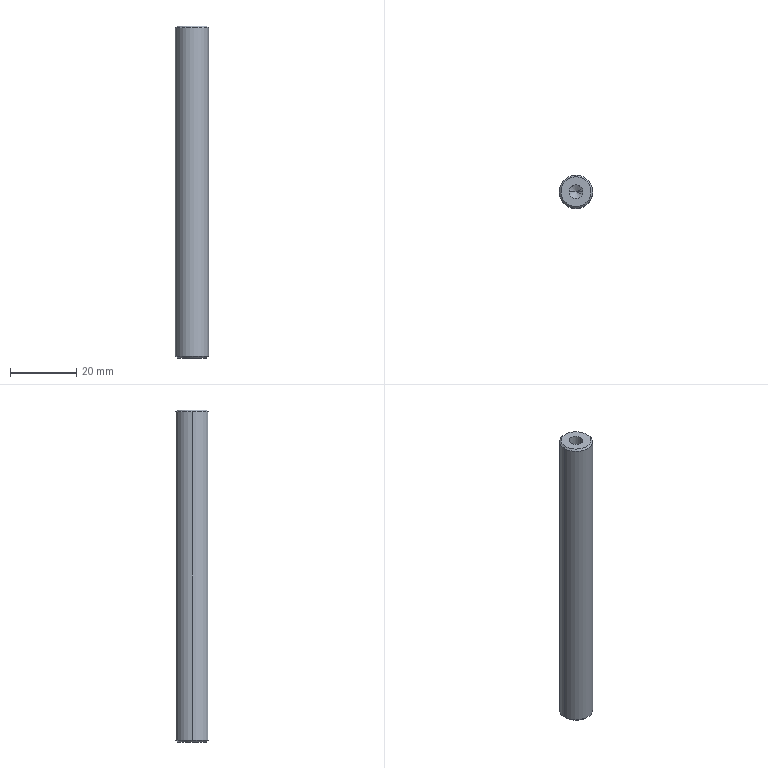Part | STEP file | 01-13 loading guide post | 1 solid | 16 faces | box 10 x 10 x 100 mm | volume 7447 mm3 | cone 8 | cylinder 6 | plane 2 | commonest cylinder face diameters 4.2 x4 10 x2
STEP:
#1=CARTESIAN_POINT('',(4.5,0.,100.));
#2=VERTEX_POINT('',#1);
#3=CARTESIAN_POINT('',(-4.5,0.,100.));
#4=VERTEX_POINT('',#3);
#5=CARTESIAN_POINT('',(0.,0.,100.));
#6=DIRECTION('',(0.,0.,1.));
#7=DIRECTION('',(1.,0.,0.));
#8=AXIS2_PLACEMENT_3D('',#5,#6,#7);
#9=CIRCLE('',#8,4.5);
#10=EDGE_CURVE('',#2,#4,#9,.T.);
#11=ORIENTED_EDGE('',*,*,#10,.F.);
#12=CARTESIAN_POINT('',(5.,0.,99.5));
#13=VERTEX_POINT('',#12);
#14=CARTESIAN_POINT('',(4.5,0.,100.));
#15=DIRECTION('',(0.7071,0.,-0.7071));
#16=VECTOR('',#15,1000.);
#17=LINE('',#14,#16);
#18=EDGE_CURVE('',#2,#13,#17,.T.);
#19=ORIENTED_EDGE('',*,*,#18,.T.);
#20=CARTESIAN_POINT('',(-5.,0.,99.5));
#21=VERTEX_POINT('',#20);
#22=CARTESIAN_POINT('',(0.,0.,99.5));
#23=DIRECTION('',(0.,0.,-1.));
#24=DIRECTION('',(1.,0.,0.));
#25=AXIS2_PLACEMENT_3D('',#22,#23,#24);
#26=CIRCLE('',#25,5.);
#27=EDGE_CURVE('',#21,#13,#26,.T.);
#28=ORIENTED_EDGE('',*,*,#27,.F.);
#29=CARTESIAN_POINT('',(-4.5,0.,100.));
#30=DIRECTION('',(-0.7071,0.,-0.7071));
#31=VECTOR('',#30,1000.);
#32=LINE('',#29,#31);
#33=EDGE_CURVE('',#4,#21,#32,.T.);
#34=ORIENTED_EDGE('',*,*,#33,.F.);
#35=EDGE_LOOP('',(#11,#19,#28,#34));
#36=FACE_OUTER_BOUND('',#35,.T.);
#37=CARTESIAN_POINT('',(0.,0.,100.));
#38=DIRECTION('',(0.,0.,-1.));
#39=DIRECTION('',(-1.,0.,0.));
#40=AXIS2_PLACEMENT_3D('',#37,#38,#39);
#41=CONICAL_SURFACE('',#40,4.5,0.7854);
#42=ADVANCED_FACE('',(#36),#41,.T.);
#43=CARTESIAN_POINT('',(-4.5,0.,0.));
#44=VERTEX_POINT('',#43);
#45=CARTESIAN_POINT('',(4.5,0.,0.));
#46=VERTEX_POINT('',#45);
#47=CARTESIAN_POINT('',(0.,0.,0.));
#48=DIRECTION('',(0.,0.,-1.));
#49=DIRECTION('',(1.,0.,0.));
#50=AXIS2_PLACEMENT_3D('',#47,#48,#49);
#51=CIRCLE('',#50,4.5);
#52=EDGE_CURVE('',#44,#46,#51,.T.);
#53=ORIENTED_EDGE('',*,*,#52,.F.);
#54=CARTESIAN_POINT('',(-5.,0.,0.5));
#55=VERTEX_POINT('',#54);
#56=CARTESIAN_POINT('',(-5.,0.,0.5));
#57=DIRECTION('',(-0.7071,0.,0.7071));
#58=VECTOR('',#57,1000.);
#59=LINE('',#56,#58);
#60=EDGE_CURVE('',#44,#55,#59,.T.);
#61=ORIENTED_EDGE('',*,*,#60,.T.);
#62=CARTESIAN_POINT('',(5.,0.,0.5));
#63=VERTEX_POINT('',#62);
#64=CARTESIAN_POINT('',(0.,0.,0.5));
#65=DIRECTION('',(0.,0.,1.));
#66=DIRECTION('',(1.,0.,0.));
#67=AXIS2_PLACEMENT_3D('',#64,#65,#66);
#68=CIRCLE('',#67,5.);
#69=EDGE_CURVE('',#63,#55,#68,.T.);
#70=ORIENTED_EDGE('',*,*,#69,.F.);
#71=CARTESIAN_POINT('',(5.,0.,0.5));
#72=DIRECTION('',(0.7071,0.,0.7071));
#73=VECTOR('',#72,1000.);
#74=LINE('',#71,#73);
#75=EDGE_CURVE('',#46,#63,#74,.T.);
#76=ORIENTED_EDGE('',*,*,#75,.F.);
#77=EDGE_LOOP('',(#53,#61,#70,#76));
#78=FACE_OUTER_BOUND('',#77,.T.);
#79=CARTESIAN_POINT('',(0.,0.,0.5));
#80=DIRECTION('',(0.,0.,1.));
#81=DIRECTION('',(1.,0.,0.));
#82=AXIS2_PLACEMENT_3D('',#79,#80,#81);
#83=CONICAL_SURFACE('',#82,5.,0.7854);
#84=ADVANCED_FACE('',(#78),#83,.T.);
#85=CARTESIAN_POINT('',(2.1,0.,14.));
#86=VERTEX_POINT('',#85);
#87=CARTESIAN_POINT('',(-2.1,0.,14.));
#88=VERTEX_POINT('',#87);
#89=CARTESIAN_POINT('',(0.,0.,14.));
#90=DIRECTION('',(0.,0.,-1.));
#91=DIRECTION('',(-1.,0.,0.));
#92=AXIS2_PLACEMENT_3D('',#89,#90,#91);
#93=CIRCLE('',#92,2.1);
#94=EDGE_CURVE('',#86,#88,#93,.T.);
#95=ORIENTED_EDGE('',*,*,#94,.F.);
#96=CARTESIAN_POINT('',(2.1,0.,0.));
#97=VERTEX_POINT('',#96);
#98=CARTESIAN_POINT('',(2.1,0.,0.));
#99=DIRECTION('',(0.,0.,-1.));
#100=VECTOR('',#99,1000.);
#101=LINE('',#98,#100);
#102=EDGE_CURVE('',#86,#97,#101,.T.);
#103=ORIENTED_EDGE('',*,*,#102,.T.);
#104=CARTESIAN_POINT('',(-2.1,0.,0.));
#105=VERTEX_POINT('',#104);
#106=CARTESIAN_POINT('',(0.,0.,0.));
#107=DIRECTION('',(0.,0.,-1.));
#108=DIRECTION('',(-1.,0.,0.));
#109=AXIS2_PLACEMENT_3D('',#106,#107,#108);
#110=CIRCLE('',#109,2.1);
#111=EDGE_CURVE('',#97,#105,#110,.T.);
#112=ORIENTED_EDGE('',*,*,#111,.T.);
#113=CARTESIAN_POINT('',(-2.1,0.,0.));
#114=DIRECTION('',(0.,0.,-1.));
#115=VECTOR('',#114,1000.);
#116=LINE('',#113,#115);
#117=EDGE_CURVE('',#88,#105,#116,.T.);
#118=ORIENTED_EDGE('',*,*,#117,.F.);
#119=EDGE_LOOP('',(#95,#103,#112,#118));
#120=FACE_OUTER_BOUND('',#119,.T.);
#121=CARTESIAN_POINT('',(0.,0.,0.));
#122=DIRECTION('',(0.,0.,-1.));
#123=DIRECTION('',(-1.,0.,0.));
#124=AXIS2_PLACEMENT_3D('',#121,#122,#123);
#125=CYLINDRICAL_SURFACE('',#124,2.1);
#126=ADVANCED_FACE('',(#120),#125,.F.);
#127=CARTESIAN_POINT('',(0.,0.,15.262));
#128=VERTEX_POINT('',#127);
#129=CARTESIAN_POINT('',(-2.1,0.,14.));
#130=DIRECTION('',(-0.8572,0.,-0.515));
#131=VECTOR('',#130,1000.);
#132=LINE('',#129,#131);
#133=EDGE_CURVE('',#128,#88,#132,.T.);
#134=ORIENTED_EDGE('',*,*,#133,.F.);
#135=CARTESIAN_POINT('',(2.1,0.,14.));
#136=DIRECTION('',(0.8572,0.,-0.515));
#137=VECTOR('',#136,1000.);
#138=LINE('',#135,#137);
#139=EDGE_CURVE('',#128,#86,#138,.T.);
#140=ORIENTED_EDGE('',*,*,#139,.T.);
#141=ORIENTED_EDGE('',*,*,#94,.T.);
#142=EDGE_LOOP('',(#134,#140,#141));
#143=FACE_OUTER_BOUND('',#142,.T.);
#144=CARTESIAN_POINT('',(0.,0.,14.));
#145=DIRECTION('',(0.,0.,-1.));
#146=DIRECTION('',(-1.,0.,0.));
#147=AXIS2_PLACEMENT_3D('',#144,#145,#146);
#148=CONICAL_SURFACE('',#147,2.1,1.03);
#149=ADVANCED_FACE('',(#143),#148,.F.);
#150=CARTESIAN_POINT('',(-2.1,0.,86.));
#151=VERTEX_POINT('',#150);
#152=CARTESIAN_POINT('',(2.1,0.,86.));
#153=VERTEX_POINT('',#152);
#154=CARTESIAN_POINT('',(0.,0.,86.));
#155=DIRECTION('',(0.,0.,1.));
#156=DIRECTION('',(1.,0.,0.));
#157=AXIS2_PLACEMENT_3D('',#154,#155,#156);
#158=CIRCLE('',#157,2.1);
#159=EDGE_CURVE('',#151,#153,#158,.T.);
#160=ORIENTED_EDGE('',*,*,#159,.F.);
#161=CARTESIAN_POINT('',(-2.1,0.,100.));
#162=VERTEX_POINT('',#161);
#163=CARTESIAN_POINT('',(-2.1,0.,100.));
#164=DIRECTION('',(0.,0.,1.));
#165=VECTOR('',#164,1000.);
#166=LINE('',#163,#165);
#167=EDGE_CURVE('',#151,#162,#166,.T.);
#168=ORIENTED_EDGE('',*,*,#167,.T.);
#169=CARTESIAN_POINT('',(2.1,0.,100.));
#170=VERTEX_POINT('',#169);
#171=CARTESIAN_POINT('',(0.,0.,100.));
#172=DIRECTION('',(0.,0.,1.));
#173=DIRECTION('',(1.,0.,0.));
#174=AXIS2_PLACEMENT_3D('',#171,#172,#173);
#175=CIRCLE('',#174,2.1);
#176=EDGE_CURVE('',#162,#170,#175,.T.);
#177=ORIENTED_EDGE('',*,*,#176,.T.);
#178=CARTESIAN_POINT('',(2.1,0.,100.));
#179=DIRECTION('',(0.,0.,1.));
#180=VECTOR('',#179,1000.);
#181=LINE('',#178,#180);
#182=EDGE_CURVE('',#153,#170,#181,.T.);
#183=ORIENTED_EDGE('',*,*,#182,.F.);
#184=EDGE_LOOP('',(#160,#168,#177,#183));
#185=FACE_OUTER_BOUND('',#184,.T.);
#186=CARTESIAN_POINT('',(0.,0.,100.));
#187=DIRECTION('',(0.,0.,1.));
#188=DIRECTION('',(1.,0.,0.));
#189=AXIS2_PLACEMENT_3D('',#186,#187,#188);
#190=CYLINDRICAL_SURFACE('',#189,2.1);
#191=ADVANCED_FACE('',(#185),#190,.F.);
#192=CARTESIAN_POINT('',(0.,0.,84.738));
#193=VERTEX_POINT('',#192);
#194=CARTESIAN_POINT('',(2.1,0.,86.));
#195=DIRECTION('',(0.8572,0.,0.515));
#196=VECTOR('',#195,1000.);
#197=LINE('',#194,#196);
#198=EDGE_CURVE('',#193,#153,#197,.T.);
#199=ORIENTED_EDGE('',*,*,#198,.F.);
#200=CARTESIAN_POINT('',(-2.1,0.,86.));
#201=DIRECTION('',(-0.8572,0.,0.515));
#202=VECTOR('',#201,1000.);
#203=LINE('',#200,#202);
#204=EDGE_CURVE('',#193,#151,#203,.T.);
#205=ORIENTED_EDGE('',*,*,#204,.T.);
#206=ORIENTED_EDGE('',*,*,#159,.T.);
#207=EDGE_LOOP('',(#199,#205,#206));
#208=FACE_OUTER_BOUND('',#207,.T.);
#209=CARTESIAN_POINT('',(0.,0.,86.));
#210=DIRECTION('',(0.,0.,1.));
#211=DIRECTION('',(1.,0.,0.));
#212=AXIS2_PLACEMENT_3D('',#209,#210,#211);
#213=CONICAL_SURFACE('',#212,2.1,1.03);
#214=ADVANCED_FACE('',(#208),#213,.F.);
#215=ORIENTED_EDGE('',*,*,#27,.T.);
#216=CARTESIAN_POINT('',(5.,0.,100.));
#217=DIRECTION('',(0.,0.,-1.));
#218=VECTOR('',#217,1000.);
#219=LINE('',#216,#218);
#220=EDGE_CURVE('',#13,#63,#219,.T.);
#221=ORIENTED_EDGE('',*,*,#220,.T.);
#222=ORIENTED_EDGE('',*,*,#69,.T.);
#223=CARTESIAN_POINT('',(-5.,0.,100.));
#224=DIRECTION('',(0.,0.,-1.));
#225=VECTOR('',#224,1000.);
#226=LINE('',#223,#225);
#227=EDGE_CURVE('',#21,#55,#226,.T.);
#228=ORIENTED_EDGE('',*,*,#227,.F.);
#229=EDGE_LOOP('',(#215,#221,#222,#228));
#230=FACE_OUTER_BOUND('',#229,.T.);
#231=CARTESIAN_POINT('',(0.,0.,100.));
#232=DIRECTION('',(0.,0.,-1.));
#233=DIRECTION('',(-1.,0.,0.));
#234=AXIS2_PLACEMENT_3D('',#231,#232,#233);
#235=CYLINDRICAL_SURFACE('',#234,5.);
#236=ADVANCED_FACE('',(#230),#235,.T.);
#237=ORIENTED_EDGE('',*,*,#220,.F.);
#238=CARTESIAN_POINT('',(0.,0.,99.5));
#239=DIRECTION('',(0.,0.,-1.));
#240=DIRECTION('',(1.,0.,0.));
#241=AXIS2_PLACEMENT_3D('',#238,#239,#240);
#242=CIRCLE('',#241,5.);
#243=EDGE_CURVE('',#13,#21,#242,.T.);
#244=ORIENTED_EDGE('',*,*,#243,.T.);
#245=ORIENTED_EDGE('',*,*,#227,.T.);
#246=CARTESIAN_POINT('',(0.,0.,0.5));
#247=DIRECTION('',(0.,0.,1.));
#248=DIRECTION('',(1.,0.,0.));
#249=AXIS2_PLACEMENT_3D('',#246,#247,#248);
#250=CIRCLE('',#249,5.);
#251=EDGE_CURVE('',#55,#63,#250,.T.);
#252=ORIENTED_EDGE('',*,*,#251,.T.);
#253=EDGE_LOOP('',(#237,#244,#245,#252));
#254=FACE_OUTER_BOUND('',#253,.T.);
#255=CARTESIAN_POINT('',(0.,0.,100.));
#256=DIRECTION('',(0.,0.,-1.));
#257=DIRECTION('',(-1.,0.,0.));
#258=AXIS2_PLACEMENT_3D('',#255,#256,#257);
#259=CYLINDRICAL_SURFACE('',#258,5.);
#260=ADVANCED_FACE('',(#254),#259,.T.);
#261=CARTESIAN_POINT('',(0.,0.,100.));
#262=DIRECTION('',(0.,0.,1.));
#263=DIRECTION('',(1.,0.,0.));
#264=AXIS2_PLACEMENT_3D('',#261,#262,#263);
#265=CIRCLE('',#264,4.5);
#266=EDGE_CURVE('',#4,#2,#265,.T.);
#267=ORIENTED_EDGE('',*,*,#266,.T.);
#268=ORIENTED_EDGE('',*,*,#10,.T.);
#269=EDGE_LOOP('',(#267,#268));
#270=FACE_OUTER_BOUND('',#269,.T.);
#271=CARTESIAN_POINT('',(0.,0.,100.));
#272=DIRECTION('',(0.,0.,1.));
#273=DIRECTION('',(1.,0.,0.));
#274=AXIS2_PLACEMENT_3D('',#271,#272,#273);
#275=CIRCLE('',#274,2.1);
#276=EDGE_CURVE('',#170,#162,#275,.T.);
#277=ORIENTED_EDGE('',*,*,#276,.F.);
#278=ORIENTED_EDGE('',*,*,#176,.F.);
#279=EDGE_LOOP('',(#277,#278));
#280=FACE_BOUND('',#279,.T.);
#281=CARTESIAN_POINT('',(0.,0.,100.));
#282=DIRECTION('',(0.,0.,1.));
#283=DIRECTION('',(1.,0.,0.));
#284=AXIS2_PLACEMENT_3D('',#281,#282,#283);
#285=PLANE('',#284);
#286=ADVANCED_FACE('',(#270,#280),#285,.T.);
#287=CARTESIAN_POINT('',(0.,0.,0.));
#288=DIRECTION('',(0.,0.,-1.));
#289=DIRECTION('',(1.,0.,0.));
#290=AXIS2_PLACEMENT_3D('',#287,#288,#289);
#291=CIRCLE('',#290,4.5);
#292=EDGE_CURVE('',#46,#44,#291,.T.);
#293=ORIENTED_EDGE('',*,*,#292,.T.);
#294=ORIENTED_EDGE('',*,*,#52,.T.);
#295=EDGE_LOOP('',(#293,#294));
#296=FACE_OUTER_BOUND('',#295,.T.);
#297=CARTESIAN_POINT('',(0.,0.,0.));
#298=DIRECTION('',(0.,0.,-1.));
#299=DIRECTION('',(-1.,0.,0.));
#300=AXIS2_PLACEMENT_3D('',#297,#298,#299);
#301=CIRCLE('',#300,2.1);
#302=EDGE_CURVE('',#105,#97,#301,.T.);
#303=ORIENTED_EDGE('',*,*,#302,.F.);
#304=ORIENTED_EDGE('',*,*,#111,.F.);
#305=EDGE_LOOP('',(#303,#304));
#306=FACE_BOUND('',#305,.T.);
#307=CARTESIAN_POINT('',(0.,0.,0.));
#308=DIRECTION('',(0.,0.,1.));
#309=DIRECTION('',(1.,0.,0.));
#310=AXIS2_PLACEMENT_3D('',#307,#308,#309);
#311=PLANE('',#310);
#312=ADVANCED_FACE('',(#296,#306),#311,.F.);
#313=ORIENTED_EDGE('',*,*,#204,.F.);
#314=ORIENTED_EDGE('',*,*,#198,.T.);
#315=CARTESIAN_POINT('',(0.,0.,86.));
#316=DIRECTION('',(0.,0.,1.));
#317=DIRECTION('',(1.,0.,0.));
#318=AXIS2_PLACEMENT_3D('',#315,#316,#317);
#319=CIRCLE('',#318,2.1);
#320=EDGE_CURVE('',#153,#151,#319,.T.);
#321=ORIENTED_EDGE('',*,*,#320,.T.);
#322=EDGE_LOOP('',(#313,#314,#321));
#323=FACE_OUTER_BOUND('',#322,.T.);
#324=CARTESIAN_POINT('',(0.,0.,86.));
#325=DIRECTION('',(0.,0.,1.));
#326=DIRECTION('',(1.,0.,0.));
#327=AXIS2_PLACEMENT_3D('',#324,#325,#326);
#328=CONICAL_SURFACE('',#327,2.1,1.03);
#329=ADVANCED_FACE('',(#323),#328,.F.);
#330=ORIENTED_EDGE('',*,*,#167,.F.);
#331=ORIENTED_EDGE('',*,*,#320,.F.);
#332=ORIENTED_EDGE('',*,*,#182,.T.);
#333=ORIENTED_EDGE('',*,*,#276,.T.);
#334=EDGE_LOOP('',(#330,#331,#332,#333));
#335=FACE_OUTER_BOUND('',#334,.T.);
#336=CARTESIAN_POINT('',(0.,0.,100.));
#337=DIRECTION('',(0.,0.,1.));
#338=DIRECTION('',(1.,0.,0.));
#339=AXIS2_PLACEMENT_3D('',#336,#337,#338);
#340=CYLINDRICAL_SURFACE('',#339,2.1);
#341=ADVANCED_FACE('',(#335),#340,.F.);
#342=ORIENTED_EDGE('',*,*,#139,.F.);
#343=ORIENTED_EDGE('',*,*,#133,.T.);
#344=CARTESIAN_POINT('',(0.,0.,14.));
#345=DIRECTION('',(0.,0.,-1.));
#346=DIRECTION('',(-1.,0.,0.));
#347=AXIS2_PLACEMENT_3D('',#344,#345,#346);
#348=CIRCLE('',#347,2.1);
#349=EDGE_CURVE('',#88,#86,#348,.T.);
#350=ORIENTED_EDGE('',*,*,#349,.T.);
#351=EDGE_LOOP('',(#342,#343,#350));
#352=FACE_OUTER_BOUND('',#351,.T.);
#353=CARTESIAN_POINT('',(0.,0.,14.));
#354=DIRECTION('',(0.,0.,-1.));
#355=DIRECTION('',(-1.,0.,0.));
#356=AXIS2_PLACEMENT_3D('',#353,#354,#355);
#357=CONICAL_SURFACE('',#356,2.1,1.03);
#358=ADVANCED_FACE('',(#352),#357,.F.);
#359=ORIENTED_EDGE('',*,*,#102,.F.);
#360=ORIENTED_EDGE('',*,*,#349,.F.);
#361=ORIENTED_EDGE('',*,*,#117,.T.);
#362=ORIENTED_EDGE('',*,*,#302,.T.);
#363=EDGE_LOOP('',(#359,#360,#361,#362));
#364=FACE_OUTER_BOUND('',#363,.T.);
#365=CARTESIAN_POINT('',(0.,0.,0.));
#366=DIRECTION('',(0.,0.,-1.));
#367=DIRECTION('',(-1.,0.,0.));
#368=AXIS2_PLACEMENT_3D('',#365,#366,#367);
#369=CYLINDRICAL_SURFACE('',#368,2.1);
#370=ADVANCED_FACE('',(#364),#369,.F.);
#371=ORIENTED_EDGE('',*,*,#60,.F.);
#372=ORIENTED_EDGE('',*,*,#292,.F.);
#373=ORIENTED_EDGE('',*,*,#75,.T.);
#374=ORIENTED_EDGE('',*,*,#251,.F.);
#375=EDGE_LOOP('',(#371,#372,#373,#374));
#376=FACE_OUTER_BOUND('',#375,.T.);
#377=CARTESIAN_POINT('',(0.,0.,0.5));
#378=DIRECTION('',(0.,0.,1.));
#379=DIRECTION('',(1.,0.,0.));
#380=AXIS2_PLACEMENT_3D('',#377,#378,#379);
#381=CONICAL_SURFACE('',#380,5.,0.7854);
#382=ADVANCED_FACE('',(#376),#381,.T.);
#383=ORIENTED_EDGE('',*,*,#18,.F.);
#384=ORIENTED_EDGE('',*,*,#266,.F.);
#385=ORIENTED_EDGE('',*,*,#33,.T.);
#386=ORIENTED_EDGE('',*,*,#243,.F.);
#387=EDGE_LOOP('',(#383,#384,#385,#386));
#388=FACE_OUTER_BOUND('',#387,.T.);
#389=CARTESIAN_POINT('',(0.,0.,100.));
#390=DIRECTION('',(0.,0.,-1.));
#391=DIRECTION('',(-1.,0.,0.));
#392=AXIS2_PLACEMENT_3D('',#389,#390,#391);
#393=CONICAL_SURFACE('',#392,4.5,0.7854);
#394=ADVANCED_FACE('',(#388),#393,.T.);
#395=CLOSED_SHELL('',(#42,#84,#126,#149,#191,#214,#236,#260,#286,#312,#329,#341,#358,#370,#382,#394));
#396=MANIFOLD_SOLID_BREP('',#395);
#397=CARTESIAN_POINT('',(0.,0.,0.));
#398=DIRECTION('',(0.,0.,1.));
#399=DIRECTION('',(1.,0.,0.));
#400=AXIS2_PLACEMENT_3D('',#397,#398,#399);
#401=(LENGTH_UNIT()NAMED_UNIT(*)SI_UNIT(.MILLI.,.METRE.));
#402=UNCERTAINTY_MEASURE_WITH_UNIT(LENGTH_MEASURE(0.00001),#401,'','');
#403=(NAMED_UNIT(*)PLANE_ANGLE_UNIT()SI_UNIT($,.RADIAN.));
#404=(NAMED_UNIT(*)SI_UNIT($,.STERADIAN.)SOLID_ANGLE_UNIT());
#405=(GEOMETRIC_REPRESENTATION_CONTEXT(3)GLOBAL_UNCERTAINTY_ASSIGNED_CONTEXT((#402))GLOBAL_UNIT_ASSIGNED_CONTEXT((#401,#403,#404))REPRESENTATION_CONTEXT('',''));
#406=ADVANCED_BREP_SHAPE_REPRESENTATION('',(#396,#400),#405);